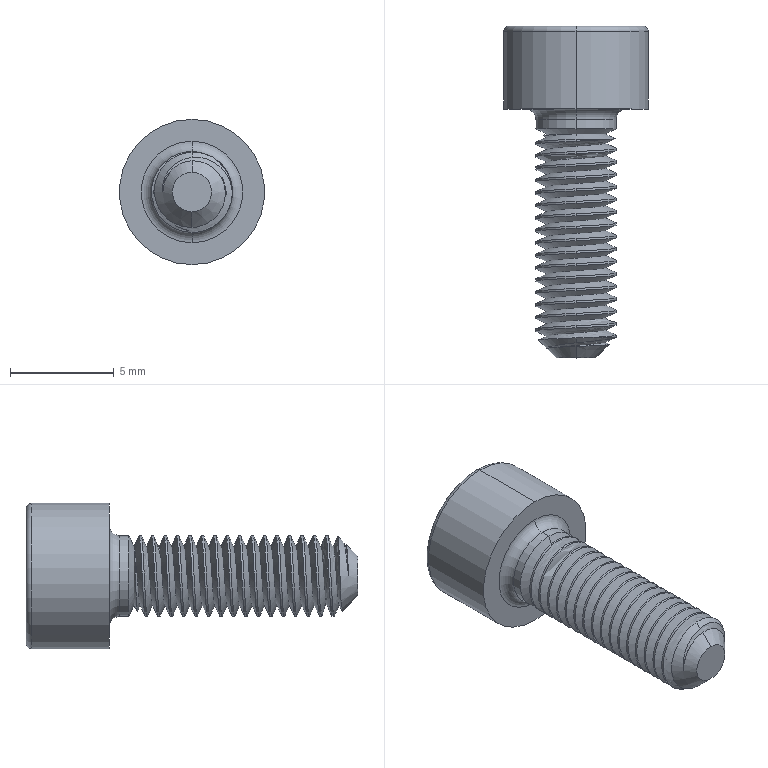Part | STEP file | Parafuso M4 - 12mm | 1 solid | 64 faces | box 7 x 16 x 7 mm | volume 239.741 mm3 | cylinder 37 | plane 10 | cone 9 | torus 6 | spline 2 | commonest cylinder face diameters 3.9 x35 7 x2